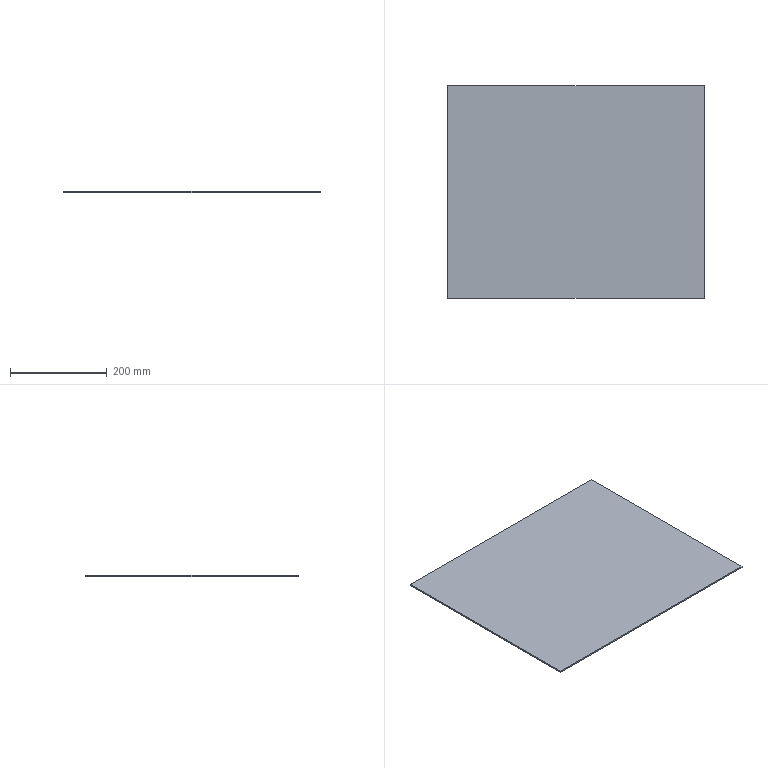Part | SolidWorks | features FlatPattern 1, SMBaseFlange 1, SheetMetal 1 | 1 solid | 6 faces | box 531 x 440 x 3 mm | volume 700920 mm3 | plane 6
STEP:
#1=CARTESIAN_POINT('',(-36.114,423.281,0.));
#2=VERTEX_POINT('',#1);
#3=CARTESIAN_POINT('',(-36.114,-16.719,0.));
#4=VERTEX_POINT('',#3);
#5=CARTESIAN_POINT('',(-36.114,-16.719,0.));
#6=DIRECTION('',(0.,-1.,0.));
#7=VECTOR('',#6,1000.);
#8=LINE('',#5,#7);
#9=EDGE_CURVE('',#2,#4,#8,.T.);
#10=ORIENTED_EDGE('',*,*,#9,.F.);
#11=CARTESIAN_POINT('',(-36.114,423.281,-3.));
#12=VERTEX_POINT('',#11);
#13=CARTESIAN_POINT('',(-36.114,423.281,-3.));
#14=DIRECTION('',(0.,0.,1.));
#15=VECTOR('',#14,1000.);
#16=LINE('',#13,#15);
#17=EDGE_CURVE('',#12,#2,#16,.T.);
#18=ORIENTED_EDGE('',*,*,#17,.F.);
#19=CARTESIAN_POINT('',(-36.114,-16.719,-3.));
#20=VERTEX_POINT('',#19);
#21=CARTESIAN_POINT('',(-36.114,-16.719,-3.));
#22=DIRECTION('',(0.,-1.,0.));
#23=VECTOR('',#22,1000.);
#24=LINE('',#21,#23);
#25=EDGE_CURVE('',#12,#20,#24,.T.);
#26=ORIENTED_EDGE('',*,*,#25,.T.);
#27=CARTESIAN_POINT('',(-36.114,-16.719,-3.));
#28=DIRECTION('',(0.,0.,1.));
#29=VECTOR('',#28,1000.);
#30=LINE('',#27,#29);
#31=EDGE_CURVE('',#20,#4,#30,.T.);
#32=ORIENTED_EDGE('',*,*,#31,.T.);
#33=EDGE_LOOP('',(#10,#18,#26,#32));
#34=FACE_OUTER_BOUND('',#33,.T.);
#35=CARTESIAN_POINT('',(-36.114,-16.719,-3.));
#36=DIRECTION('',(-1.,0.,0.));
#37=DIRECTION('',(0.,0.,1.));
#38=AXIS2_PLACEMENT_3D('',#35,#36,#37);
#39=PLANE('',#38);
#40=ADVANCED_FACE('',(#34),#39,.T.);
#41=CARTESIAN_POINT('',(494.886,423.281,0.));
#42=VERTEX_POINT('',#41);
#43=CARTESIAN_POINT('',(-36.114,423.281,0.));
#44=DIRECTION('',(-1.,0.,0.));
#45=VECTOR('',#44,1000.);
#46=LINE('',#43,#45);
#47=EDGE_CURVE('',#42,#2,#46,.T.);
#48=ORIENTED_EDGE('',*,*,#47,.F.);
#49=CARTESIAN_POINT('',(494.886,423.281,-3.));
#50=VERTEX_POINT('',#49);
#51=CARTESIAN_POINT('',(494.886,423.281,-3.));
#52=DIRECTION('',(0.,0.,1.));
#53=VECTOR('',#52,1000.);
#54=LINE('',#51,#53);
#55=EDGE_CURVE('',#50,#42,#54,.T.);
#56=ORIENTED_EDGE('',*,*,#55,.F.);
#57=CARTESIAN_POINT('',(-36.114,423.281,-3.));
#58=DIRECTION('',(-1.,0.,0.));
#59=VECTOR('',#58,1000.);
#60=LINE('',#57,#59);
#61=EDGE_CURVE('',#50,#12,#60,.T.);
#62=ORIENTED_EDGE('',*,*,#61,.T.);
#63=ORIENTED_EDGE('',*,*,#17,.T.);
#64=EDGE_LOOP('',(#48,#56,#62,#63));
#65=FACE_OUTER_BOUND('',#64,.T.);
#66=CARTESIAN_POINT('',(-36.114,423.281,-3.));
#67=DIRECTION('',(0.,1.,0.));
#68=DIRECTION('',(0.,0.,1.));
#69=AXIS2_PLACEMENT_3D('',#66,#67,#68);
#70=PLANE('',#69);
#71=ADVANCED_FACE('',(#65),#70,.T.);
#72=CARTESIAN_POINT('',(494.886,-16.719,0.));
#73=VERTEX_POINT('',#72);
#74=CARTESIAN_POINT('',(494.886,-16.719,0.));
#75=DIRECTION('',(0.,1.,0.));
#76=VECTOR('',#75,1000.);
#77=LINE('',#74,#76);
#78=EDGE_CURVE('',#73,#42,#77,.T.);
#79=ORIENTED_EDGE('',*,*,#78,.F.);
#80=CARTESIAN_POINT('',(494.886,-16.719,-3.));
#81=VERTEX_POINT('',#80);
#82=CARTESIAN_POINT('',(494.886,-16.719,-3.));
#83=DIRECTION('',(0.,0.,1.));
#84=VECTOR('',#83,1000.);
#85=LINE('',#82,#84);
#86=EDGE_CURVE('',#81,#73,#85,.T.);
#87=ORIENTED_EDGE('',*,*,#86,.F.);
#88=CARTESIAN_POINT('',(494.886,-16.719,-3.));
#89=DIRECTION('',(0.,1.,0.));
#90=VECTOR('',#89,1000.);
#91=LINE('',#88,#90);
#92=EDGE_CURVE('',#81,#50,#91,.T.);
#93=ORIENTED_EDGE('',*,*,#92,.T.);
#94=ORIENTED_EDGE('',*,*,#55,.T.);
#95=EDGE_LOOP('',(#79,#87,#93,#94));
#96=FACE_OUTER_BOUND('',#95,.T.);
#97=CARTESIAN_POINT('',(494.886,-16.719,-3.));
#98=DIRECTION('',(1.,0.,0.));
#99=DIRECTION('',(0.,0.,-1.));
#100=AXIS2_PLACEMENT_3D('',#97,#98,#99);
#101=PLANE('',#100);
#102=ADVANCED_FACE('',(#96),#101,.T.);
#103=CARTESIAN_POINT('',(-36.114,-16.719,0.));
#104=DIRECTION('',(1.,0.,0.));
#105=VECTOR('',#104,1000.);
#106=LINE('',#103,#105);
#107=EDGE_CURVE('',#4,#73,#106,.T.);
#108=ORIENTED_EDGE('',*,*,#107,.F.);
#109=ORIENTED_EDGE('',*,*,#31,.F.);
#110=CARTESIAN_POINT('',(-36.114,-16.719,-3.));
#111=DIRECTION('',(1.,0.,0.));
#112=VECTOR('',#111,1000.);
#113=LINE('',#110,#112);
#114=EDGE_CURVE('',#20,#81,#113,.T.);
#115=ORIENTED_EDGE('',*,*,#114,.T.);
#116=ORIENTED_EDGE('',*,*,#86,.T.);
#117=EDGE_LOOP('',(#108,#109,#115,#116));
#118=FACE_OUTER_BOUND('',#117,.T.);
#119=CARTESIAN_POINT('',(-36.114,-16.719,-3.));
#120=DIRECTION('',(0.,-1.,0.));
#121=DIRECTION('',(0.,0.,-1.));
#122=AXIS2_PLACEMENT_3D('',#119,#120,#121);
#123=PLANE('',#122);
#124=ADVANCED_FACE('',(#118),#123,.T.);
#125=ORIENTED_EDGE('',*,*,#25,.F.);
#126=ORIENTED_EDGE('',*,*,#61,.F.);
#127=ORIENTED_EDGE('',*,*,#92,.F.);
#128=ORIENTED_EDGE('',*,*,#114,.F.);
#129=EDGE_LOOP('',(#125,#126,#127,#128));
#130=FACE_OUTER_BOUND('',#129,.T.);
#131=CARTESIAN_POINT('',(0.,0.,-3.));
#132=DIRECTION('',(0.,0.,-1.));
#133=DIRECTION('',(-1.,0.,0.));
#134=AXIS2_PLACEMENT_3D('',#131,#132,#133);
#135=PLANE('',#134);
#136=ADVANCED_FACE('',(#130),#135,.T.);
#137=ORIENTED_EDGE('',*,*,#9,.T.);
#138=ORIENTED_EDGE('',*,*,#107,.T.);
#139=ORIENTED_EDGE('',*,*,#78,.T.);
#140=ORIENTED_EDGE('',*,*,#47,.T.);
#141=EDGE_LOOP('',(#137,#138,#139,#140));
#142=FACE_OUTER_BOUND('',#141,.T.);
#143=CARTESIAN_POINT('',(0.,0.,0.));
#144=DIRECTION('',(0.,0.,-1.));
#145=DIRECTION('',(-1.,0.,0.));
#146=AXIS2_PLACEMENT_3D('',#143,#144,#145);
#147=PLANE('',#146);
#148=ADVANCED_FACE('',(#142),#147,.F.);
#149=CLOSED_SHELL('',(#40,#71,#102,#124,#136,#148));
#150=MANIFOLD_SOLID_BREP('',#149);
#151=CARTESIAN_POINT('',(0.,0.,0.));
#152=DIRECTION('',(0.,0.,1.));
#153=DIRECTION('',(1.,0.,0.));
#154=AXIS2_PLACEMENT_3D('',#151,#152,#153);
#155=(LENGTH_UNIT()NAMED_UNIT(*)SI_UNIT(.MILLI.,.METRE.));
#156=UNCERTAINTY_MEASURE_WITH_UNIT(LENGTH_MEASURE(0.00001),#155,'','');
#157=(NAMED_UNIT(*)PLANE_ANGLE_UNIT()SI_UNIT($,.RADIAN.));
#158=(NAMED_UNIT(*)SI_UNIT($,.STERADIAN.)SOLID_ANGLE_UNIT());
#159=(GEOMETRIC_REPRESENTATION_CONTEXT(3)GLOBAL_UNCERTAINTY_ASSIGNED_CONTEXT((#156))GLOBAL_UNIT_ASSIGNED_CONTEXT((#155,#157,#158))REPRESENTATION_CONTEXT('',''));
#160=ADVANCED_BREP_SHAPE_REPRESENTATION('',(#150,#154),#159);